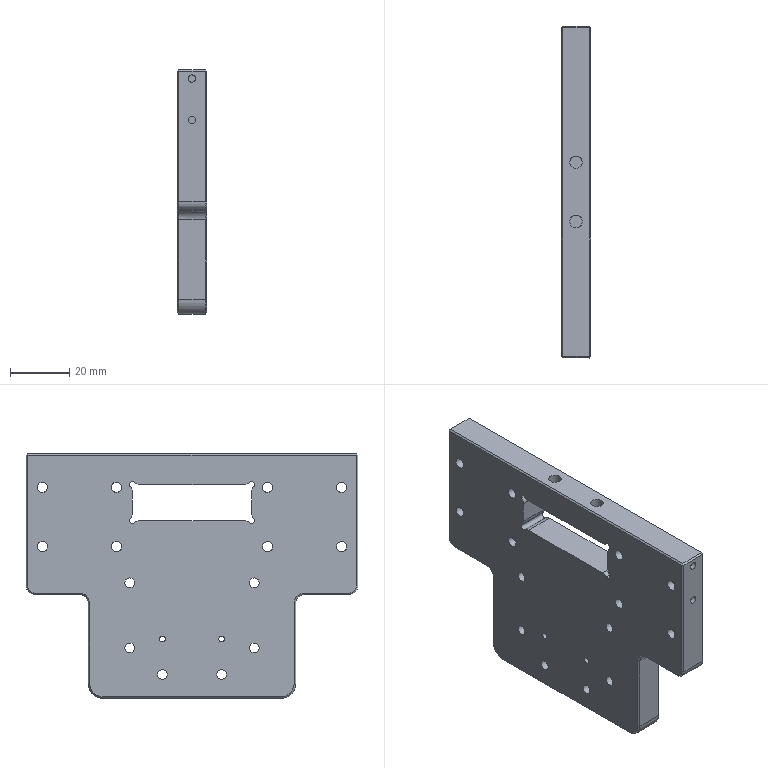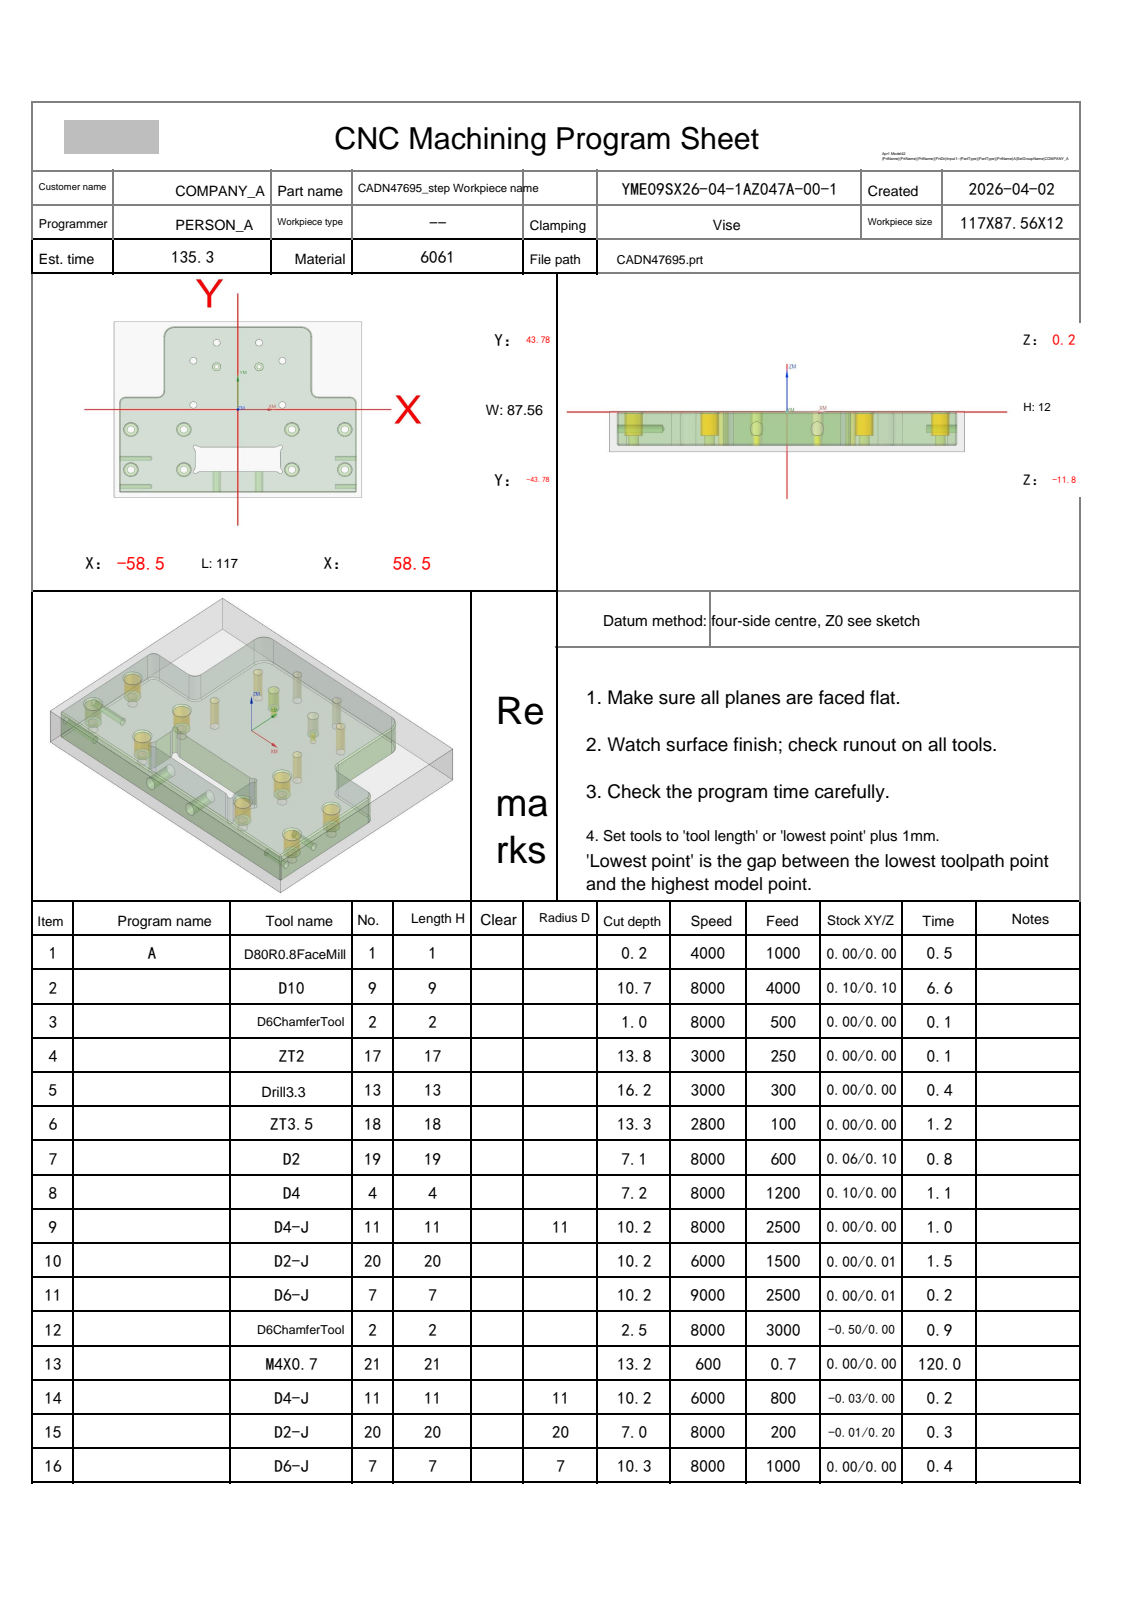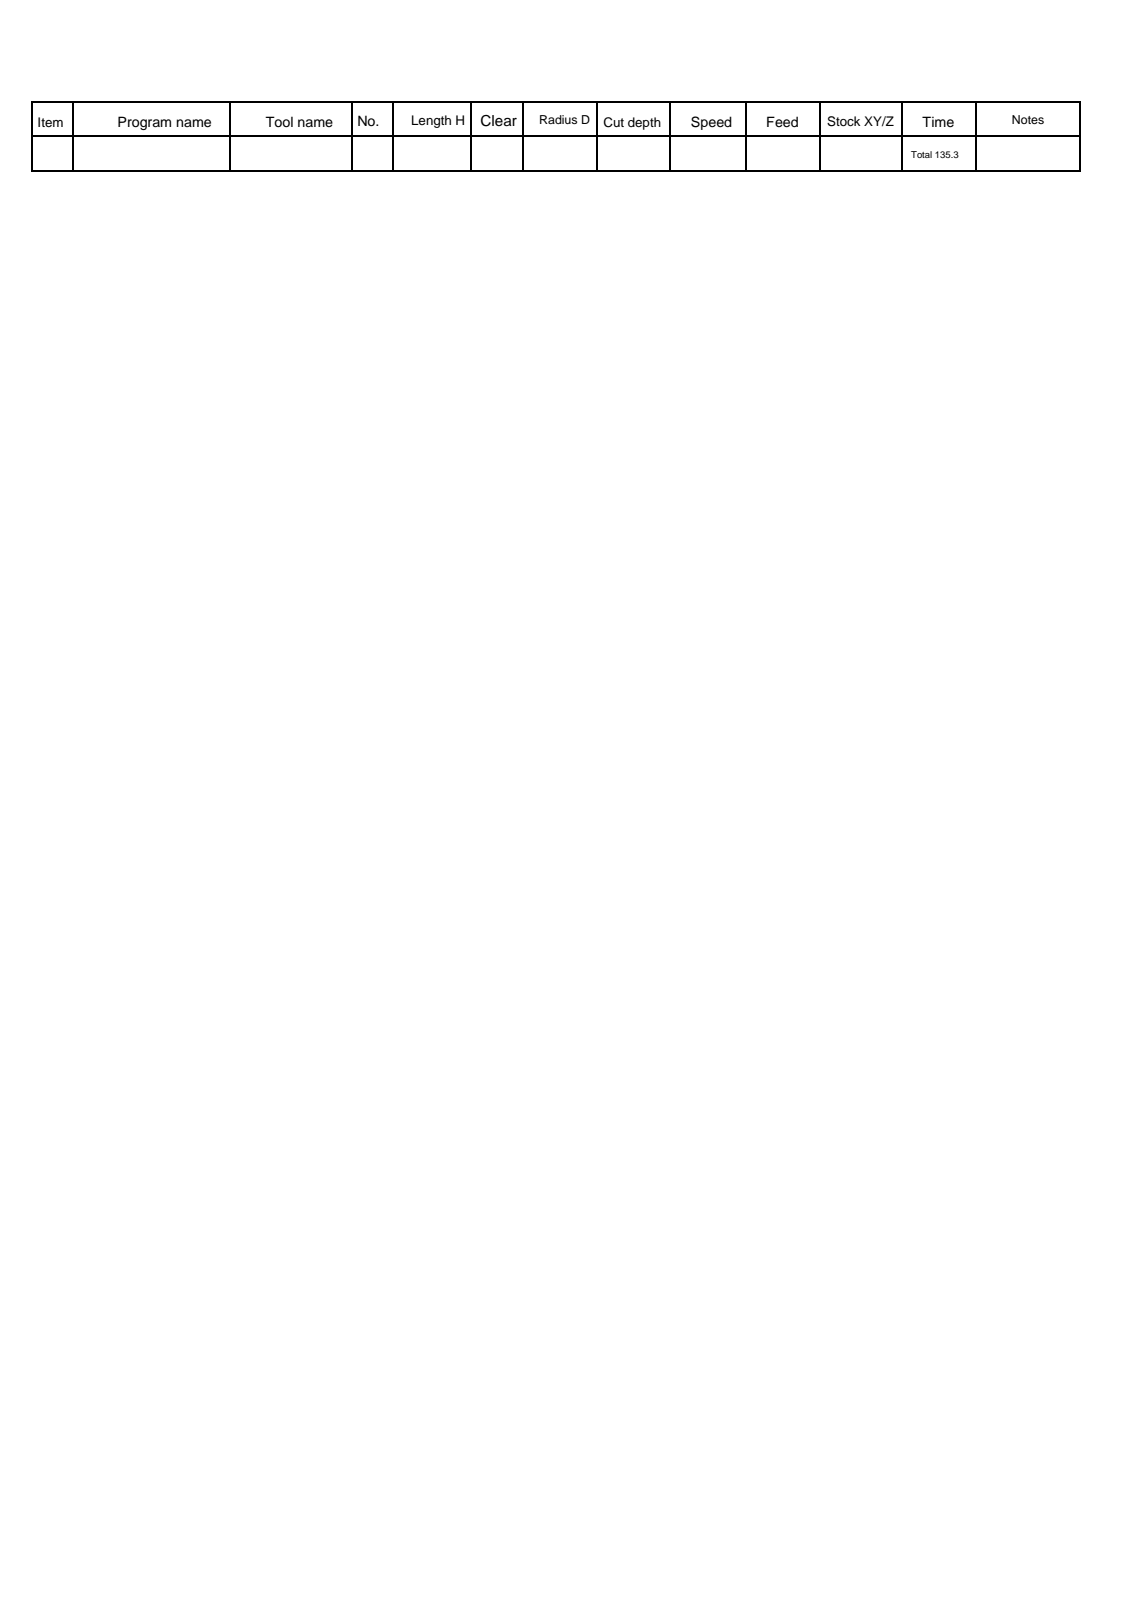NC program | NX | posted by the shop | part box 10 x 112 x 82.562 mm
Lines 41 to 1171 of 16718:
N2 T09 M06
(D10  D=10. R=0. H=09 ce=0.10 di=0.10)
G00 G90 G54 X-70.5 Y18.03 M03 S8000
G43 H09 Z10.2
M08
Z.719
G01 Z-.481 F4000.
X-66.
G03 X-59. Y25.03 I0.0 J7.
G01 Y43.781
G02 X-58.5 Y44.281 I.5 J0.0
G01 X-38.251
G02 X-29.994 Y47.779 I8.257 J-7.996
G01 X-29.952
X29.96
X29.968
G02 X38.24 Y44.281 I0.0 J-11.53
G01 X58.5
G02 X59. Y43.781 I0.0 J-.5
G01 Y13.777
G02 X58. Y12.777 I-1. J0.0
G01 X57.833 Y12.791
X52.819 Y13.639
X52.652 Y13.652
G03 X51.826 Y13.216 I0.0 J-1.
G02 X51.002 Y12.779 I-.826 J.563
G01 X42.496
G02 X41.498 Y13.777 I.002 J1.
G01 Y36.281
G02 X42.496 Y37.281 I1. J0.0
G01 X51.002
G02 X52. Y36.284 I-.002 J-1.
G01 Y17.242
G02 X51.2 Y16.442 I-.8 J0.0
G01 X51.051 Y16.456
X46.766 Y17.266
X46.65 Y17.281
G02 X45.998 Y17.977 I.048 J.698
G01 Y32.084
G02 X46.696 Y32.781 I.7 J-.002
G01 X46.802
G02 X47.5 Y32.084 I-.002 J-.7
G01 Y20.327
G03 X47.689 Y19.742 I1. J0.0
G01 X51.636 Y14.281
G03 X52.446 Y13.867 I.81 J.586
G01 X52.613 Y13.88
X57.833 Y14.763
X58. Y14.777
G02 X59. Y13.777 I0.0 J-1.
G01 Y10.644
G02 X62.498 Y3.281 I-6. J-7.363
G01 Y-40.781
G02 X60.595 Y-45.376 I-6.498 J0.0
G01 X60.095 Y-45.876
G02 X55.5 Y-47.779 I-4.595 J4.595
G01 X-55.5
G02 X-60.095 Y-45.876 I0.0 J6.498
G01 X-60.595 Y-45.376
G02 X-62.498 Y-40.781 I4.595 J4.595
G01 Y3.281
G02 X-59. Y10.644 I9.498 J0.0
G01 Y30.03
G02 X-58.238 Y31.002 I1. J0.0
G01 X-52.762 Y32.344
G03 X-52. Y33.315 I-.238 J.971
G01 Y36.284
G02 X-51.002 Y37.281 I1. J-.002
G01 X-42.496
G02 X-41.499 Y36.289 I-.002 J-1.
G01 X-41.498 Y32.781
Y13.777
G02 X-42.496 Y12.779 I-1. J.002
G01 X-50.51
G03 X-51.214 Y12.334 I0.0 J-.779
G01 X-51.382 Y11.979
X-51.422 Y11.799
G03 X-51.002 Y11.379 I.42 J0.0
G01 X-40.098
Y36.281
X-40.13 Y36.378
X-40.063 Y36.455
X-40.068 Y36.928
G02 X-29.994 Y46.379 I10.074 J-.643
G01 X-29.955
X29.961
X29.968
G02 X40.098 Y36.256 I0.0 J-10.13
G01 Y11.379
X53.039
G02 X61.098 Y3.281 I-.039 J-8.098
G01 Y-40.781
G02 X59.605 Y-44.386 I-5.098 J0.0
G01 X59.105 Y-44.886
G02 X55.5 Y-46.379 I-3.605 J3.605
G01 X-55.5
G02 X-59.105 Y-44.886 I0.0 J5.098
G01 X-59.605 Y-44.386
G02 X-61.098 Y-40.781 I3.605 J3.605
G01 Y3.281
G02 X-53.039 Y11.379 I8.098 J0.0
G01 X-51.002
G03 X-50.582 Y11.799 I0.0 J.42
G01 X-50.623 Y11.979
X-50.906 Y12.577
G03 X-51.191 Y12.798 I-.361 J-.172
G02 X-52. Y13.777 I.191 J.982
G01 Y27.364
G02 X-51.705 Y28.073 I1. J0.0
G01 X-47.613 Y32.138
G03 X-47.425 Y32.396 I-.705 J.709
G02 X-46.802 Y32.781 I.625 J-.315
G01 X-46.696
G02 X-45.998 Y32.084 I-.002 J-.7
G01 Y17.977
G02 X-46.696 Y17.279 I-.7 J.002
G01 X-46.802
G02 X-47.5 Y17.977 I.002 J.7
G01 Y30.03
Y30.53
G03 X-54.5 Y37.53 I-7. J0.0
G01 X-70.5
Z.719
G00 Z3.
G01 Y18.031 F6000.
G00 Z.238
G01 Z-.962 F4000.
X-66.
G03 X-59. Y25.031 I0.0 J7.
G01 Y43.781
G02 X-58.5 Y44.281 I.5 J0.0
G01 X-38.262
G02 X-30.001 Y47.781 I8.261 J-8.
G01 X30.001
G02 X38.255 Y44.281 I-.012 J-11.511
G01 X58.5
G02 X59. Y43.781 I0.0 J-.5
G01 Y13.778
G02 X58. Y12.778 I-1. J0.0
G01 X57.833 Y12.792
X52.818 Y13.64
X52.652 Y13.654
G03 X51.826 Y13.218 I0.0 J-1.
G02 X51.003 Y12.781 I-.826 J.563
G01 X42.497
G02 X41.5 Y13.778 I.003 J1.
G01 Y36.284
G02 X42.497 Y37.281 I1. J-.003
G01 X51.003
G02 X52. Y36.284 I-.003 J-1.
G01 Y17.244
G02 X51.2 Y16.444 I-.8 J0.0
G01 X51.051 Y16.458
X46.767 Y17.268
X46.651 Y17.283
G02 X46. Y17.979 I.048 J.698
G01 Y32.084
G02 X46.697 Y32.781 I.7 J-.003
G01 X46.803
G02 X47.5 Y32.084 I-.003 J-.7
G01 Y20.329
G03 X47.689 Y19.743 I1. J0.0
G01 X51.636 Y14.282
G03 X52.446 Y13.868 I.81 J.586
G01 X52.613 Y13.882
X57.833 Y14.764
X58. Y14.778
G02 X59. Y13.778 I0.0 J-1.
G01 Y10.647
G02 X62.5 Y3.281 I-6. J-7.365
G01 Y-40.781
G02 X60.596 Y-45.377 I-6.5 J0.0
G01 X60.096 Y-45.877
G02 X55.5 Y-47.781 I-4.596 J4.596
G01 X-55.5
G02 X-60.096 Y-45.877 I0.0 J6.5
G01 X-60.596 Y-45.377
G02 X-62.5 Y-40.781 I4.596 J4.596
G01 Y3.281
G02 X-59. Y10.647 I9.5 J0.0
G01 Y30.031
G02 X-58.238 Y31.002 I1. J0.0
G01 X-52.762 Y32.345
G03 X-52. Y33.315 I-.238 J.971
G01 Y36.284
G02 X-51.003 Y37.281 I1. J-.003
G01 X-42.498
G02 X-41.5 Y36.284 I-.003 J-1.
G01 Y13.778
G02 X-42.498 Y12.781 I-1. J.003
G01 X-50.51
G03 X-51.214 Y12.336 I0.0 J-.779
G01 X-51.382 Y11.981
X-51.423 Y11.801
G03 X-51.003 Y11.381 I.42 J0.0
G01 X-40.1
Y36.281
G02 X-30.001 Y46.381 I10.1 J0.0
G01 X30.
G02 X40.1 Y36.31 I-.011 J-10.111
G01 Y11.381
X53.
G02 X61.1 Y3.281 I0.0 J-8.1
G01 Y-40.781
G02 X59.606 Y-44.387 I-5.1 J0.0
G01 X59.106 Y-44.887
G02 X55.5 Y-46.381 I-3.606 J3.606
G01 X-55.5
G02 X-59.106 Y-44.887 I0.0 J5.1
G01 X-59.606 Y-44.387
G02 X-61.1 Y-40.781 I3.606 J3.606
G01 Y3.281
G02 X-53. Y11.381 I8.1 J0.0
G01 X-52.949
X-51.003
G03 X-50.583 Y11.801 I0.0 J.42
G01 X-50.623 Y11.981
X-50.907 Y12.579
G03 X-51.191 Y12.8 I-.361 J-.172
G02 X-52. Y13.778 I.191 J.982
G01 Y27.365
G02 X-51.705 Y28.074 I1. J0.0
G01 X-47.612 Y32.139
G03 X-47.425 Y32.397 I-.705 J.709
G02 X-46.803 Y32.781 I.625 J-.316
G01 X-46.698
G02 X-46. Y32.084 I-.003 J-.7
G01 Y17.979
G02 X-46.698 Y17.281 I-.7 J.003
G01 X-46.803
G02 X-47.5 Y17.979 I.003 J.7
G01 Y30.031
Y30.531
G03 X-54.5 Y37.531 I-7. J0.0
G01 X-70.5
Z.238
G00 Z2.519
G01 Y18.031 F6000.
G00 Z-.243
G01 Z-1.443 F4000.
X-66.
G03 X-59. Y25.031 I0.0 J7.
G01 Y43.781
G02 X-58.5 Y44.281 I.5 J0.0
G01 X-38.262
G02 X-30.001 Y47.781 I8.261 J-8.
G01 X30.001
G02 X38.255 Y44.281 I-.012 J-11.511
G01 X58.5
G02 X59. Y43.781 I0.0 J-.5
G01 Y13.778
G02 X58. Y12.778 I-1. J0.0
G01 X57.833 Y12.792
X52.818 Y13.64
X52.652 Y13.654
G03 X51.826 Y13.218 I0.0 J-1.
G02 X51.003 Y12.781 I-.826 J.563
G01 X42.497
G02 X41.5 Y13.778 I.003 J1.
G01 Y36.284
G02 X42.497 Y37.281 I1. J-.003
G01 X51.003
G02 X52. Y36.284 I-.003 J-1.
G01 Y17.244
G02 X51.2 Y16.444 I-.8 J0.0
G01 X51.051 Y16.458
X46.767 Y17.268
X46.651 Y17.283
G02 X46. Y17.979 I.048 J.698
G01 Y32.084
G02 X46.697 Y32.781 I.7 J-.003
G01 X46.803
G02 X47.5 Y32.084 I-.003 J-.7
G01 Y20.329
G03 X47.689 Y19.743 I1. J0.0
G01 X51.636 Y14.282
G03 X52.446 Y13.868 I.81 J.586
G01 X52.613 Y13.882
X57.833 Y14.764
X58. Y14.778
G02 X59. Y13.778 I0.0 J-1.
G01 Y10.647
G02 X62.5 Y3.281 I-6. J-7.365
G01 Y-40.781
G02 X60.596 Y-45.377 I-6.5 J0.0
G01 X60.096 Y-45.877
G02 X55.5 Y-47.781 I-4.596 J4.596
G01 X-55.5
G02 X-60.096 Y-45.877 I0.0 J6.5
G01 X-60.596 Y-45.377
G02 X-62.5 Y-40.781 I4.596 J4.596
G01 Y3.281
G02 X-59. Y10.647 I9.5 J0.0
G01 Y30.031
G02 X-58.238 Y31.002 I1. J0.0
G01 X-52.762 Y32.345
G03 X-52. Y33.315 I-.238 J.971
G01 Y36.284
G02 X-51.003 Y37.281 I1. J-.003
G01 X-42.498
G02 X-41.501 Y36.284 I-.003 J-1.
G01 Y13.778
G02 X-42.498 Y12.781 I-1. J.003
G01 X-50.511
G03 X-51.214 Y12.336 I0.0 J-.779
G01 X-51.382 Y11.981
X-51.423 Y11.801
G03 X-51.003 Y11.381 I.42 J0.0
G01 X-40.101
Y36.281
G02 X-30.001 Y46.381 I10.1 J0.0
G01 X30.
G02 X40.1 Y36.31 I-.011 J-10.111
G01 Y11.381
X53.
G02 X61.1 Y3.281 I0.0 J-8.1
G01 Y-40.781
G02 X59.606 Y-44.387 I-5.1 J0.0
G01 X59.106 Y-44.887
G02 X55.5 Y-46.381 I-3.606 J3.606
G01 X-55.5
G02 X-59.106 Y-44.887 I0.0 J5.1
G01 X-59.606 Y-44.387
G02 X-61.1 Y-40.781 I3.606 J3.606
G01 Y3.281
G02 X-53. Y11.381 I8.1 J0.0
G01 X-52.949
X-51.003
G03 X-50.583 Y11.801 I0.0 J.42
G01 X-50.623 Y11.981
X-50.907 Y12.579
G03 X-51.191 Y12.8 I-.361 J-.172
G02 X-52. Y13.778 I.191 J.982
G01 Y27.365
G02 X-51.705 Y28.074 I1. J0.0
G01 X-47.612 Y32.139
G03 X-47.425 Y32.397 I-.705 J.709
G02 X-46.803 Y32.781 I.625 J-.316
G01 X-46.698
G02 X-46.001 Y32.084 I-.003 J-.7
G01 Y17.979
G02 X-46.698 Y17.281 I-.7 J.003
G01 X-46.803
G02 X-47.5 Y17.979 I.003 J.7
G01 Y30.031
Y30.531
G03 X-54.5 Y37.531 I-7. J0.0
G01 X-70.5
Z-.243
G00 Z2.038
G01 Y18.031 F6000.
G00 Z-.724
G01 Z-1.924 F4000.
X-66.
G03 X-59. Y25.031 I0.0 J7.
G01 Y43.781
G02 X-58.5 Y44.281 I.5 J0.0
G01 X-38.263
G02 X-30.002 Y47.781 I8.261 J-8.
G01 X30.001
X30.144 Y47.78
G02 X38.255 Y44.281 I-.155 J-11.51
G01 X58.5
G02 X59. Y43.781 I0.0 J-.5
G01 Y13.778
G02 X58. Y12.778 I-1. J0.0
G01 X57.833 Y12.792
X52.818 Y13.64
X52.652 Y13.653
G03 X51.826 Y13.218 I0.0 J-1.
G02 X51.003 Y12.781 I-.826 J.564
G01 X42.496
G02 X41.5 Y13.778 I.003 J1.
G01 Y36.285
G02 X42.496 Y37.281 I1. J-.003
G01 X51.003
G02 X52. Y36.285 I-.003 J-1.
G01 Y17.243
G02 X51.2 Y16.443 I-.8 J0.0
G01 X51.051 Y16.457
X46.767 Y17.268
X46.651 Y17.283
G02 X46. Y17.978 I.049 J.698
G01 Y32.084
G02 X46.697 Y32.781 I.7 J-.003
G01 X46.803
G02 X47.5 Y32.084 I-.003 J-.7
G01 Y20.328
G03 X47.689 Y19.743 I1. J0.0
G01 X51.636 Y14.282
G03 X52.446 Y13.867 I.81 J.586
G01 X52.613 Y13.881
X57.833 Y14.764
X58. Y14.778
G02 X59. Y13.778 I0.0 J-1.
G01 Y10.647
G02 X62.5 Y3.281 I-6. J-7.365
G01 Y-40.781
G02 X60.596 Y-45.377 I-6.5 J0.0
G01 X60.096 Y-45.877
G02 X55.5 Y-47.781 I-4.596 J4.596
G01 X-55.5
G02 X-60.096 Y-45.877 I0.0 J6.5
G01 X-60.596 Y-45.377
G02 X-62.5 Y-40.781 I4.596 J4.596
G01 Y3.281
G02 X-59. Y10.647 I9.5 J0.0
G01 Y30.031
G02 X-58.238 Y31.002 I1. J0.0
G01 X-52.762 Y32.345
G03 X-52. Y33.315 I-.238 J.971
G01 Y36.285
G02 X-51.003 Y37.281 I1. J-.003
G01 X-42.498
G02 X-41.501 Y36.284 I-.003 J-1.
G01 Y13.778
G02 X-42.498 Y12.781 I-1. J.003
G01 X-50.511
G03 X-51.214 Y12.336 I0.0 J-.779
G01 X-51.383 Y11.981
X-51.423 Y11.801
G03 X-51.003 Y11.381 I.42 J0.0
G01 X-40.101
Y36.281
G02 X-30.002 Y46.381 I10.1 J0.0
G01 X30.
X30.125 Y46.38
G02 X40.1 Y36.31 I-.136 J-10.11
G01 Y11.381
X53.
G02 X61.1 Y3.281 I0.0 J-8.1
G01 Y-40.781
G02 X59.606 Y-44.387 I-5.1 J0.0
G01 X59.106 Y-44.887
G02 X55.5 Y-46.381 I-3.606 J3.606
G01 X-55.5
G02 X-59.106 Y-44.887 I0.0 J5.1
G01 X-59.606 Y-44.387
G02 X-61.1 Y-40.781 I3.606 J3.606
G01 Y3.281
G02 X-53. Y11.381 I8.1 J0.0
G01 X-52.949
X-51.003
G03 X-50.583 Y11.801 I0.0 J.42
G01 X-50.624 Y11.981
X-50.907 Y12.579
G03 X-51.192 Y12.8 I-.361 J-.172
G02 X-52. Y13.778 I.192 J.981
G01 Y27.365
G02 X-51.705 Y28.074 I1. J0.0
G01 X-47.612 Y32.139
G03 X-47.425 Y32.397 I-.705 J.709
G02 X-46.803 Y32.781 I.625 J-.316
G01 X-46.698
G02 X-46.001 Y32.084 I-.003 J-.7
G01 Y17.978
G02 X-46.698 Y17.281 I-.7 J.003
G01 X-46.803
G02 X-47.5 Y17.978 I.003 J.7
G01 Y30.031
Y30.531
G03 X-54.5 Y37.531 I-7. J0.0
G01 X-70.5
Z-.724
G00 Z1.557
G01 Y18.031 F6000.
G00 Z-1.205
G01 Z-2.405 F4000.
X-66.
G03 X-59. Y25.031 I0.0 J7.
G01 Y43.781
G02 X-58.5 Y44.281 I.5 J0.0
G01 X-38.263
G02 X-30.002 Y47.781 I8.261 J-8.
G01 X30.001
X30.135 Y47.78
G02 X38.255 Y44.281 I-.146 J-11.51
G01 X58.5
G02 X59. Y43.781 I0.0 J-.5
G01 Y13.778
G02 X58. Y12.778 I-1. J0.0
G01 X57.833 Y12.792
X52.818 Y13.639
X52.652 Y13.653
G03 X51.826 Y13.217 I0.0 J-1.
G02 X51.004 Y12.781 I-.826 J.564
G01 X42.496
G02 X41.5 Y13.778 I.004 J1.
G01 Y36.285
G02 X42.496 Y37.281 I1. J-.004
G01 X51.004
G02 X52. Y36.285 I-.004 J-1.
G01 Y17.243
G02 X51.2 Y16.443 I-.8 J0.0
G01 X51.051 Y16.457
X46.767 Y17.268
X46.651 Y17.283
G02 X46. Y17.978 I.049 J.698
G01 Y32.084
G02 X46.697 Y32.781 I.7 J-.003
G01 X46.803
G02 X47.5 Y32.084 I-.003 J-.7
G01 Y20.328
G03 X47.689 Y19.743 I1. J0.0
G01 X51.636 Y14.281
G03 X52.446 Y13.867 I.81 J.586
G01 X52.613 Y13.881
X57.833 Y14.764
X58. Y14.778
G02 X59. Y13.778 I0.0 J-1.
G01 Y10.647
G02 X62.5 Y3.281 I-6. J-7.365
G01 Y-40.781
G02 X60.596 Y-45.377 I-6.5 J0.0
G01 X60.096 Y-45.877
G02 X55.5 Y-47.781 I-4.596 J4.596
G01 X-55.5
G02 X-60.096 Y-45.877 I0.0 J6.5
G01 X-60.596 Y-45.377
G02 X-62.5 Y-40.781 I4.596 J4.596
G01 Y3.281
G02 X-59. Y10.647 I9.5 J0.0
G01 Y30.031
G02 X-58.238 Y31.002 I1. J0.0
G01 X-52.762 Y32.345
G03 X-52. Y33.315 I-.238 J.971
G01 Y36.285
G02 X-51.004 Y37.281 I1. J-.004
G01 X-42.498
G02 X-41.501 Y36.285 I-.004 J-1.
G01 Y13.778
G02 X-42.498 Y12.781 I-1. J.004
G01 X-50.511
G03 X-51.215 Y12.336 I0.0 J-.779
G01 X-51.383 Y11.981
X-51.424 Y11.801
G03 X-51.004 Y11.381 I.42 J0.0
G01 X-40.101
Y36.281
G02 X-30.002 Y46.381 I10.1 J0.0
G01 X30.118 Y46.38
G02 X40.1 Y36.31 I-.128 J-10.11
G01 Y11.381
X53.
G02 X61.1 Y3.281 I0.0 J-8.1
G01 Y-40.781
G02 X59.606 Y-44.387 I-5.1 J0.0
G01 X59.106 Y-44.887
G02 X55.5 Y-46.381 I-3.606 J3.606
G01 X-55.5
G02 X-59.106 Y-44.887 I0.0 J5.1
G01 X-59.606 Y-44.387
G02 X-61.1 Y-40.781 I3.606 J3.606
G01 Y3.281
G02 X-53. Y11.381 I8.1 J0.0
G01 X-52.949
X-51.004
G03 X-50.584 Y11.801 I0.0 J.42
G01 X-50.624 Y11.981
X-50.908 Y12.579
G03 X-51.192 Y12.8 I-.361 J-.172
G02 X-52. Y13.778 I.192 J.981
G01 Y27.365
G02 X-51.705 Y28.074 I1. J0.0
G01 X-47.612 Y32.139
G03 X-47.425 Y32.397 I-.705 J.709
G02 X-46.803 Y32.781 I.625 J-.316
G01 X-46.698
G02 X-46.001 Y32.084 I-.003 J-.7
G01 Y17.978
G02 X-46.698 Y17.281 I-.7 J.003
G01 X-46.803
G02 X-47.5 Y17.978 I.003 J.7
G01 Y30.031
Y30.531
G03 X-54.5 Y37.531 I-7. J0.0
G01 X-70.5
Z-1.205
G00 Z1.076
G01 Y18.031 F6000.
G00 Z-1.686
G01 Z-2.886 F4000.
X-66.
G03 X-59. Y25.031 I0.0 J7.
G01 Y43.781
G02 X-58.5 Y44.281 I.5 J0.0
G01 X-38.263
G02 X-30.002 Y47.781 I8.261 J-8.
G01 X30.001
X30.132 Y47.78
G02 X38.255 Y44.281 I-.143 J-11.51
G01 X58.5
G02 X59. Y43.781 I0.0 J-.5
G01 Y13.778
G02 X58. Y12.778 I-1. J0.0
G01 X57.833 Y12.792
X52.818 Y13.639
X52.652 Y13.653
G03 X51.826 Y13.217 I0.0 J-1.
G02 X51.004 Y12.781 I-.826 J.564
G01 X42.496
G02 X41.5 Y13.778 I.004 J1.
G01 Y36.285
G02 X42.496 Y37.281 I1. J-.004
G01 X51.004
G02 X52. Y36.285 I-.004 J-1.
G01 Y17.243
G02 X51.2 Y16.443 I-.8 J0.0
G01 X51.051 Y16.457
X46.767 Y17.268
X46.651 Y17.283
G02 X46. Y17.978 I.049 J.698
G01 Y32.084
G02 X46.697 Y32.781 I.7 J-.003
G01 X46.803
G02 X47.5 Y32.084 I-.003 J-.7
G01 Y20.328
G03 X47.689 Y19.743 I1. J0.0
G01 X51.636 Y14.281
G03 X52.446 Y13.867 I.81 J.586
G01 X52.613 Y13.881
X57.833 Y14.764
X58. Y14.778
G02 X59. Y13.778 I0.0 J-1.
G01 Y10.647
G02 X62.5 Y3.281 I-6. J-7.365
G01 Y-40.781
G02 X60.596 Y-45.377 I-6.5 J0.0
G01 X60.096 Y-45.877
G02 X55.5 Y-47.781 I-4.596 J4.596
G01 X-55.5
G02 X-60.096 Y-45.877 I0.0 J6.5
G01 X-60.596 Y-45.377
G02 X-62.5 Y-40.781 I4.596 J4.596
G01 Y3.281
G02 X-59. Y10.647 I9.5 J0.0
G01 Y30.031
G02 X-58.238 Y31.002 I1. J0.0
G01 X-52.762 Y32.345
G03 X-52. Y33.315 I-.238 J.971
G01 Y36.285
G02 X-51.004 Y37.281 I1. J-.004
G01 X-42.498
G02 X-41.502 Y36.285 I-.004 J-1.
G01 Y13.778
G02 X-42.498 Y12.781 I-1. J.004
G01 X-50.511
G03 X-51.215 Y12.336 I0.0 J-.779
G01 X-51.383 Y11.981
X-51.424 Y11.801
G03 X-51.004 Y11.381 I.42 J0.0
G01 X-40.102
Y36.281
G02 X-30.002 Y46.381 I10.1 J0.0
G01 X30.115 Y46.38
G02 X40.1 Y36.31 I-.125 J-10.11
G01 Y11.381
X53.
G02 X61.1 Y3.281 I0.0 J-8.1
G01 Y-40.781
G02 X59.606 Y-44.387 I-5.1 J0.0
G01 X59.106 Y-44.887
G02 X55.5 Y-46.381 I-3.606 J3.606
G01 X-55.5
G02 X-59.106 Y-44.887 I0.0 J5.1
G01 X-59.606 Y-44.387
G02 X-61.1 Y-40.781 I3.606 J3.606
G01 Y3.281
G02 X-53. Y11.381 I8.1 J0.0
G01 X-52.949
X-51.004
G03 X-50.584 Y11.801 I0.0 J.42
G01 X-50.624 Y11.981
X-50.908 Y12.579
G03 X-51.192 Y12.8 I-.361 J-.172
G02 X-52. Y13.778 I.192 J.981
G01 Y27.365
G02 X-51.705 Y28.074 I1. J0.0
G01 X-47.612 Y32.139
G03 X-47.425 Y32.397 I-.705 J.709
G02 X-46.803 Y32.781 I.625 J-.316
G01 X-46.699
G02 X-46.002 Y32.084 I-.003 J-.7
G01 Y17.978
G02 X-46.699 Y17.281 I-.7 J.003
G01 X-46.803
G02 X-47.5 Y17.978 I.003 J.7
G01 Y30.031
Y30.531
G03 X-54.5 Y37.531 I-7. J0.0
G01 X-70.5
Z-1.686
G00 Z.595
G01 Y18.031 F6000.
G00 Z-2.167
G01 Z-3.367 F4000.
X-66.
G03 X-59. Y25.031 I0.0 J7.
G01 Y43.781
G02 X-58.5 Y44.281 I.5 J0.0
G01 X-38.264
G02 X-30.003 Y47.781 I8.261 J-8.
G01 X30.001
X30.129 Y47.78
G02 X38.255 Y44.281 I-.14 J-11.51
G01 X58.5
G02 X59. Y43.781 I0.0 J-.5
G01 Y13.777
G02 X58. Y12.777 I-1. J0.0
G01 X57.833 Y12.791
X52.818 Y13.639
X52.651 Y13.653
G03 X51.826 Y13.217 I0.0 J-1.
G02 X51.004 Y12.781 I-.826 J.564
G01 X42.496
G02 X41.5 Y13.777 I.004 J1.
G01 Y36.285
G02 X42.496 Y37.281 I1. J-.004
G01 X51.004
G02 X52. Y36.285 I-.004 J-1.
G01 Y17.243
G02 X51.2 Y16.443 I-.8 J0.0
G01 X51.051 Y16.457
X46.766 Y17.268
X46.651 Y17.283
G02 X46. Y17.978 I.049 J.698
G01 Y32.085
G02 X46.696 Y32.781 I.7 J-.003
G01 X46.803
G02 X47.5 Y32.085 I-.003 J-.7
G01 Y20.328
G03 X47.689 Y19.743 I1. J0.0
G01 X51.636 Y14.281
G03 X52.446 Y13.867 I.81 J.586
G01 X52.613 Y13.881
X57.833 Y14.763
X58. Y14.777
G02 X59. Y13.777 I0.0 J-1.
G01 Y10.647
G02 X62.5 Y3.281 I-6. J-7.365
G01 Y-40.781
G02 X60.596 Y-45.377 I-6.5 J0.0
G01 X60.096 Y-45.877
G02 X55.5 Y-47.781 I-4.596 J4.596
G01 X-55.5
G02 X-60.096 Y-45.877 I0.0 J6.5
G01 X-60.596 Y-45.377
G02 X-62.5 Y-40.781 I4.596 J4.596
G01 Y3.281
G02 X-59. Y10.647 I9.5 J0.0
G01 Y30.031
G02 X-58.238 Y31.002 I1. J0.0
G01 X-52.762 Y32.345
G03 X-52. Y33.315 I-.238 J.971
G01 Y36.285
G02 X-51.004 Y37.281 I1. J-.004
G01 X-42.498
G02 X-41.502 Y36.285 I-.004 J-1.
G01 Y13.777
G02 X-42.498 Y12.781 I-1. J.004
G01 X-50.511
G03 X-51.215 Y12.336 I0.0 J-.779
G01 X-51.383 Y11.981
X-51.424 Y11.801
G03 X-51.004 Y11.381 I.42 J0.0
G01 X-40.102
Y36.281
G02 X-30.003 Y46.381 I10.1 J0.0
G01 X30.112 Y46.38
G02 X40.1 Y36.31 I-.123 J-10.11
G01 Y11.381
X53.
G02 X61.1 Y3.281 I0.0 J-8.1
G01 Y-40.781
G02 X59.606 Y-44.387 I-5.1 J0.0
G01 X59.106 Y-44.887
G02 X55.5 Y-46.381 I-3.606 J3.606
G01 X-55.5
G02 X-59.106 Y-44.887 I0.0 J5.1
G01 X-59.606 Y-44.387
G02 X-61.1 Y-40.781 I3.606 J3.606
G01 Y3.281
G02 X-53. Y11.381 I8.1 J0.0
G01 X-52.949
X-51.004
G03 X-50.584 Y11.801 I0.0 J.42
G01 X-50.624 Y11.981
X-50.908 Y12.579
G03 X-51.192 Y12.8 I-.361 J-.172
G02 X-52. Y13.777 I.192 J.981
G01 Y27.365
G02 X-51.705 Y28.074 I1. J0.0
G01 X-47.612 Y32.139
G03 X-47.425 Y32.397 I-.705 J.709
G02 X-46.803 Y32.781 I.625 J-.316
G01 X-46.699
G02 X-46.002 Y32.085 I-.003 J-.7
G01 Y17.978
G02 X-46.699 Y17.281 I-.7 J.003
G01 X-46.803
G02 X-47.5 Y17.978 I.003 J.7
G01 Y30.031
Y30.531
G03 X-54.5 Y37.531 I-7. J0.0
G01 X-70.5
Z-2.167
G00 Z.114
G01 Y18.031 F6000.
G00 Z-2.648
G01 Z-3.848 F4000.
X-66.
G03 X-59. Y25.031 I0.0 J7.
G01 Y43.781
G02 X-58.5 Y44.281 I.5 J0.0
G01 X-38.264
G02 X-30.003 Y47.781 I8.261 J-8.
G01 X30.001
X30.124 Y47.78
G02 X38.255 Y44.281 I-.135 J-11.51
G01 X58.5
G02 X59. Y43.781 I0.0 J-.5
G01 Y13.777
G02 X58. Y12.777 I-1. J0.0
G01 X57.833 Y12.791
X52.818 Y13.639
X52.651 Y13.653
G03 X51.826 Y13.217 I0.0 J-1.
G02 X51.004 Y12.781 I-.826 J.564
G01 X42.496
G02 X41.5 Y13.777 I.004 J1.
G01 Y36.285
G02 X42.496 Y37.281 I1. J-.004
G01 X51.004
G02 X52. Y36.285 I-.004 J-1.
G01 Y17.243
G02 X51.2 Y16.443 I-.8 J0.0
G01 X51.051 Y16.457
X46.766 Y17.268
X46.651 Y17.283
G02 X46. Y17.978 I.049 J.698
G01 Y32.085
G02 X46.696 Y32.781 I.7 J-.004
G01 X46.804
G02 X47.5 Y32.085 I-.004 J-.7
G01 Y20.328
G03 X47.689 Y19.743 I1. J0.0
G01 X51.636 Y14.281
G03 X52.446 Y13.867 I.81 J.586
G01 X52.613 Y13.881
X57.833 Y14.763
X58. Y14.777
G02 X59. Y13.777 I0.0 J-1.
G01 Y10.647
G02 X62.5 Y3.281 I-6. J-7.365
G01 Y-40.781
G02 X60.596 Y-45.377 I-6.5 J0.0
G01 X60.096 Y-45.877
G02 X55.5 Y-47.781 I-4.596 J4.596
G01 X-55.5
G02 X-60.096 Y-45.877 I0.0 J6.5
G01 X-60.596 Y-45.377
G02 X-62.5 Y-40.781 I4.596 J4.596
G01 Y3.281
G02 X-59. Y10.647 I9.5 J0.0
G01 Y30.031
G02 X-58.238 Y31.002 I1. J0.0
G01 X-52.762 Y32.345
G03 X-52. Y33.315 I-.238 J.971
G01 Y36.285
G02 X-51.004 Y37.281 I1. J-.004
G01 X-42.498
G02 X-41.502 Y36.285 I-.004 J-1.
G01 Y13.777
G02 X-42.498 Y12.781 I-1. J.004
G01 X-50.512
G03 X-51.215 Y12.336 I0.0 J-.779
G01 X-51.383 Y11.981
X-51.424 Y11.801
G03 X-51.004 Y11.381 I.42 J0.0
G01 X-40.102
Y36.281
G02 X-30.003 Y46.381 I10.1 J0.0
G01 X30.108
G02 X40.1 Y36.31 I-.119 J-10.11
G01 Y11.381
X53.
G02 X61.1 Y3.281 I0.0 J-8.1
G01 Y-40.781
G02 X59.606 Y-44.387 I-5.1 J0.0
G01 X59.106 Y-44.887
G02 X55.5 Y-46.381 I-3.606 J3.606
G01 X-55.5
G02 X-59.106 Y-44.887 I0.0 J5.1
G01 X-59.606 Y-44.387
G02 X-61.1 Y-40.781 I3.606 J3.606
G01 Y3.281
G02 X-53. Y11.381 I8.1 J0.0
G01 X-52.949
X-51.004
G03 X-50.584 Y11.801 I0.0 J.42
G01 X-50.625 Y11.981
X-50.908 Y12.579
G03 X-51.192 Y12.8 I-.361 J-.172
G02 X-52. Y13.777 I.192 J.981
G01 Y27.365
G02 X-51.705 Y28.074 I1. J0.0
G01 X-47.612 Y32.139
G03 X-47.425 Y32.397 I-.705 J.709
G02 X-46.804 Y32.781 I.625 J-.316
G01 X-46.699
G02 X-46.002 Y32.085 I-.004 J-.7
G01 Y17.978
G02 X-46.699 Y17.281 I-.7 J.004
G01 X-46.804
G02 X-47.5 Y17.978 I.004 J.7
G01 Y30.031
Y30.531
G03 X-54.5 Y37.531 I-7. J0.0
G01 X-70.5
Z-2.648
G00 Z-.367
G01 Y18.031 F6000.
G00 Z-3.129
G01 Z-4.329 F4000.
X-66.
G03 X-59. Y25.031 I0.0 J7.
G01 Y43.781
G02 X-58.5 Y44.281 I.5 J0.0
G01 X-38.264
G02 X-30.003 Y47.781 I8.261 J-8.
G01 X30.119 Y47.78
G02 X38.255 Y44.281 I-.13 J-11.51
G01 X58.5
G02 X59. Y43.781 I0.0 J-.5
G01 Y13.777
G02 X58. Y12.777 I-1. J0.0
G01 X57.833 Y12.791
X52.818 Y13.639
X52.651 Y13.653
G03 X51.826 Y13.217 I0.0 J-1.
G02 X51.004 Y12.781 I-.826 J.564
G01 X42.496
G02 X41.5 Y13.777 I.004 J1.
G01 Y36.285
G02 X42.496 Y37.281 I1. J-.004
G01 X51.004
G02 X52. Y36.285 I-.004 J-1.
G01 Y17.243
G02 X51.2 Y16.443 I-.8 J0.0
G01 X51.051 Y16.457
X46.766 Y17.268
X46.651 Y17.283
G02 X46. Y17.978 I.049 J.698
G01 Y32.085
G02 X46.696 Y32.781 I.7 J-.004
G01 X46.804
G02 X47.5 Y32.085 I-.004 J-.7
G01 Y20.328
G03 X47.689 Y19.743 I1. J0.0
G01 X51.636 Y14.281
G03 X52.446 Y13.867 I.81 J.586
G01 X52.613 Y13.881
X57.833 Y14.763
X58. Y14.777
G02 X59. Y13.777 I0.0 J-1.
G01 Y10.647
G02 X62.5 Y3.281 I-6. J-7.365
G01 Y-40.781
G02 X60.596 Y-45.377 I-6.5 J0.0
G01 X60.096 Y-45.877
G02 X55.5 Y-47.781 I-4.596 J4.596
G01 X-55.5
G02 X-60.096 Y-45.877 I0.0 J6.5
G01 X-60.596 Y-45.377
G02 X-62.5 Y-40.781 I4.596 J4.596
G01 Y3.281
G02 X-59. Y10.647 I9.5 J0.0
G01 Y30.031
G02 X-58.238 Y31.002 I1. J0.0
G01 X-52.762 Y32.345
G03 X-52. Y33.315 I-.238 J.971
G01 Y36.285
G02 X-51.004 Y37.281 I1. J-.004
G01 X-42.499
G02 X-41.503 Y36.285 I-.004 J-1.
G01 Y13.777
G02 X-42.499 Y12.781 I-1. J.004
G01 X-50.512
G03 X-51.215 Y12.336 I0.0 J-.779
G01 X-51.384 Y11.981
X-51.424 Y11.801
G03 X-51.004 Y11.381 I.42 J0.0
G01 X-40.103
Y36.281
G02 X-30.003 Y46.381 I10.1 J0.0
G01 X30.103
G02 X40.1 Y36.31 I-.114 J-10.11
G01 Y11.381
X53.
G02 X61.1 Y3.281 I0.0 J-8.1
G01 Y-40.781
G02 X59.606 Y-44.387 I-5.1 J0.0
G01 X59.106 Y-44.887
G02 X55.5 Y-46.381 I-3.606 J3.606
G01 X-55.5
G02 X-59.106 Y-44.887 I0.0 J5.1
G01 X-59.606 Y-44.387
G02 X-61.1 Y-40.781 I3.606 J3.606
G01 Y3.281
G02 X-53. Y11.381 I8.1 J0.0
G01 X-52.949
X-51.004
G03 X-50.584 Y11.801 I0.0 J.42
G01 X-50.625 Y11.981
X-50.908 Y12.579
G03 X-51.192 Y12.8 I-.361 J-.172
G02 X-52. Y13.777 I.192 J.981
G01 Y27.365
G02 X-51.705 Y28.074 I1. J0.0
G01 X-47.612 Y32.139
G03 X-47.425 Y32.397 I-.705 J.709
G02 X-46.804 Y32.781 I.625 J-.316
G01 X-46.699
G02 X-46.003 Y32.085 I-.004 J-.7
G01 Y17.978
G02 X-46.699 Y17.281 I-.7 J.004
G01 X-46.804
G02 X-47.5 Y17.978 I.004 J.7
G01 Y30.031
Y30.531
G03 X-54.5 Y37.531 I-7. J0.0
G01 X-70.5
Z-3.129
G00 Z-.848
G01 Y18.031 F6000.
G00 Z-3.61
G01 Z-4.81 F4000.
X-66.
G03 X-59. Y25.031 I0.0 J7.
G01 Y43.781
G02 X-58.5 Y44.281 I.5 J0.0
G01 X-38.265
G02 X-30.004 Y47.781 I8.261 J-8.
G01 X30.115
G02 X38.255 Y44.281 I-.126 J-11.51
G01 X58.5
G02 X59. Y43.781 I0.0 J-.5
G01 Y13.777
G02 X58. Y12.777 I-1. J0.0
G01 X57.833 Y12.791
X52.818 Y13.639
X52.651 Y13.653
G03 X51.826 Y13.217 I0.0 J-1.
G02 X51.004 Y12.781 I-.826 J.564
G01 X42.496
G02 X41.5 Y13.777 I.004 J1.
G01 Y36.286
G02 X42.496 Y37.281 I1. J-.004
G01 X51.004
G02 X52. Y36.286 I-.004 J-1.
G01 Y17.243
G02 X51.2 Y16.443 I-.8 J0.0
G01 X51.051 Y16.457
X46.766 Y17.268
X46.651 Y17.283
G02 X46. Y17.977 I.049 J.698
G01 Y32.085
G02 X46.696 Y32.781 I.7 J-.004
G01 X46.804
G02 X47.5 Y32.085 I-.004 J-.7
G01 Y20.328
G03 X47.689 Y19.743 I1. J0.0
G01 X51.636 Y14.281
G03 X52.446 Y13.867 I.81 J.586
G01 X52.613 Y13.88
X57.833 Y14.763
X58. Y14.777
G02 X59. Y13.777 I0.0 J-1.
G01 Y10.647
G02 X62.5 Y3.281 I-6. J-7.365
G01 Y-40.781
G02 X60.596 Y-45.377 I-6.5 J0.0
G01 X60.096 Y-45.877
G02 X55.5 Y-47.781 I-4.596 J4.596
G01 X-55.5
G02 X-60.096 Y-45.877 I0.0 J6.5
G01 X-60.596 Y-45.377
G02 X-62.5 Y-40.781 I4.596 J4.596
G01 Y3.281
G02 X-59. Y10.647 I9.5 J0.0
G01 Y30.031
G02 X-58.238 Y31.002 I1. J0.0
G01 X-52.762 Y32.345
G03 X-52. Y33.315 I-.238 J.971
G01 Y36.286
G02 X-51.004 Y37.281 I1. J-.004
G01 X-42.499
G02 X-41.503 Y36.285 I-.004 J-1.
G01 Y13.777
G02 X-42.499 Y12.781 I-1. J.004
G01 X-50.512
G03 X-51.215 Y12.336 I0.0 J-.779
G01 X-51.384 Y11.981
X-51.424 Y11.801
G03 X-51.004 Y11.381 I.42 J0.0
G01 X-40.103
Y36.281
G02 X-30.004 Y46.381 I10.1 J0.0
G01 X30.1
G02 X40.1 Y36.31 I-.11 J-10.11
G01 Y11.381
X53.
G02 X61.1 Y3.281 I0.0 J-8.1
G01 Y-40.781
G02 X59.606 Y-44.387 I-5.1 J0.0
G01 X59.106 Y-44.887
G02 X55.5 Y-46.381 I-3.606 J3.606
G01 X-55.5
G02 X-59.106 Y-44.887 I0.0 J5.1
G01 X-59.606 Y-44.387
G02 X-61.1 Y-40.781 I3.606 J3.606
G01 Y3.281
G02 X-53. Y11.381 I8.1 J0.0
G01 X-52.949
X-51.004
G03 X-50.584 Y11.801 I0.0 J.42
G01 X-50.625 Y11.981
X-50.908 Y12.579
G03 X-51.192 Y12.8 I-.361 J-.172
G02 X-52. Y13.777 I.192 J.981
G01 Y27.365